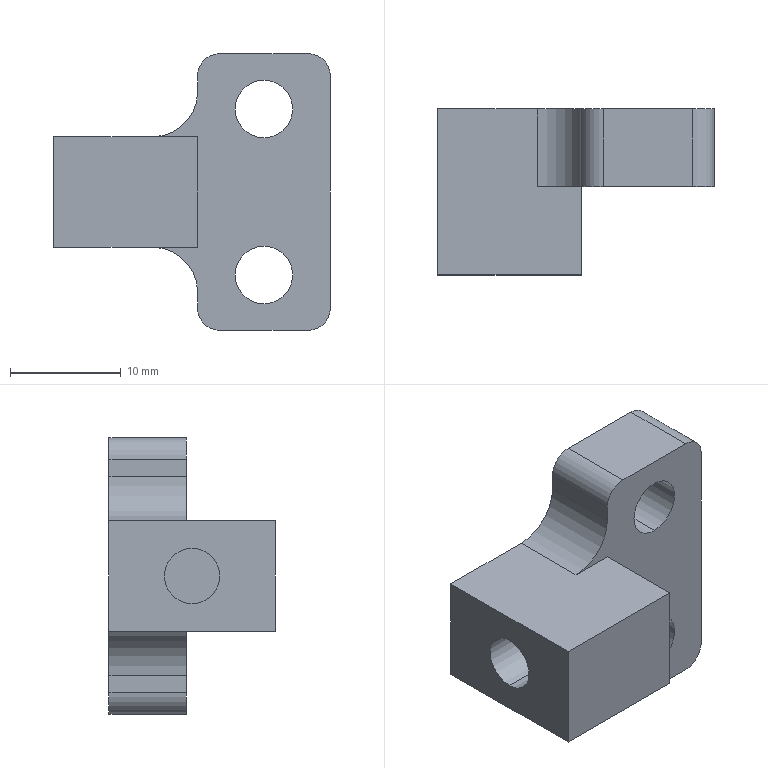Part | 1 solid | 25 faces | volume 3541 mm3 | plane 13 | cylinder 12 | commonest cylinder face diameters 4 x4 5.2 x4 5 x2 8 x2